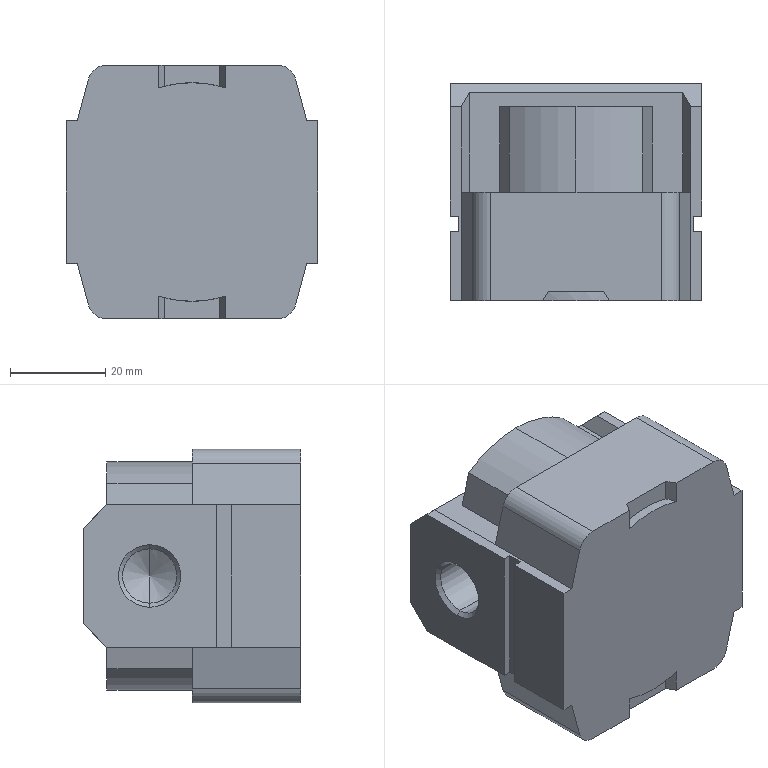Part | STEP file | _AF30-02-A(0)_BODY | 1 solid | 97 faces | box 53 x 45.8 x 53.4 mm | volume 97884 mm3 | plane 52 | cone 24 | cylinder 21 | commonest cylinder face diameters 3.242 x8 8 x4 11.445 x4 48 x3 46 x2